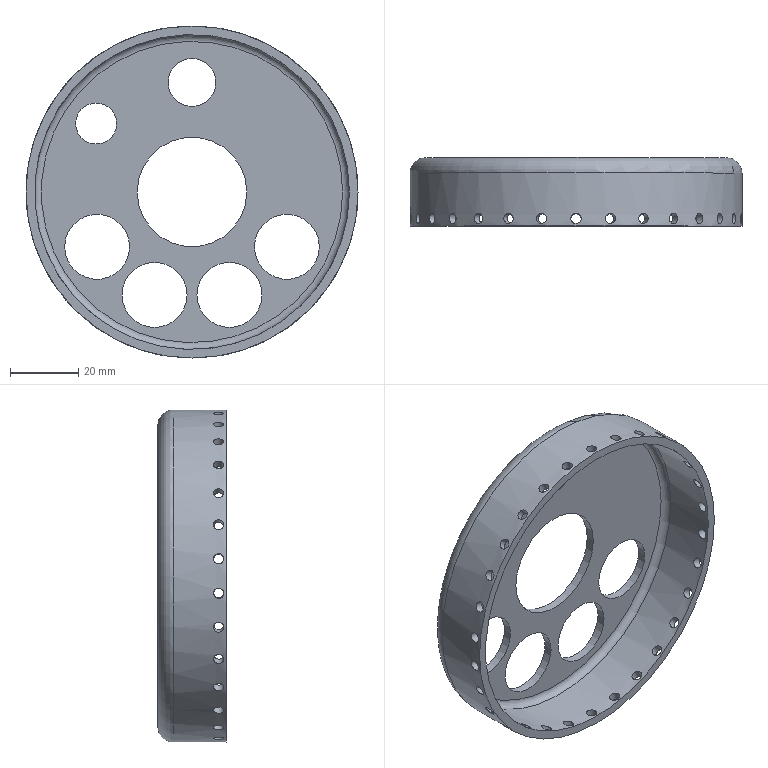Part | STEP file | 1-56.3 | 1 solid | 44 faces | box 97 x 20 x 97 mm | volume 24368 mm3 | cylinder 39 | plane 3 | torus 2 | commonest cylinder face diameters 3 x30 19 x4 12 x1 14 x1 32 x1 92 x1